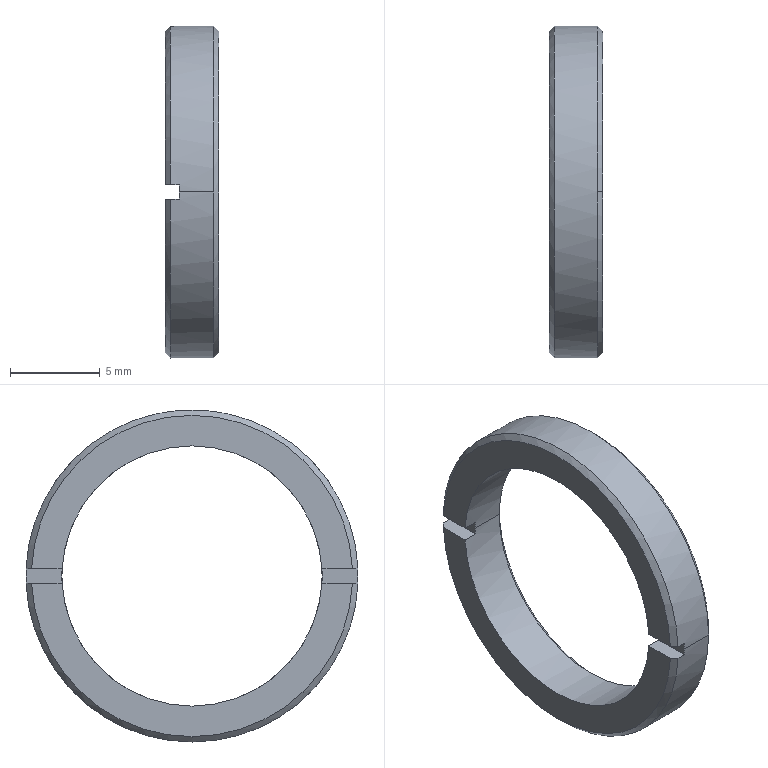Part | STEP file | pressure ring 3.stp.STEP-214.STEP | 1 solid | 20 faces | box 3 x 18.5 x 18.5 mm | volume 301.276 mm3 | plane 9 | cone 7 | cylinder 4 | commonest cylinder face diameters 14.5 x2 18.5 x2
STEP:
#1=CARTESIAN_POINT('',(427.54,0.,7.25));
#2=VERTEX_POINT('',#1);
#3=CARTESIAN_POINT('',(427.54,-7.25,0.));
#4=VERTEX_POINT('',#3);
#5=CARTESIAN_POINT('',(427.54,0.,0.));
#6=DIRECTION('',(1.,0.,0.));
#7=DIRECTION('',(0.,0.,1.));
#8=AXIS2_PLACEMENT_3D('',#5,#6,#7);
#9=CIRCLE('',#8,7.25);
#10=EDGE_CURVE('',#2,#4,#9,.T.);
#11=ORIENTED_EDGE('',*,*,#10,.T.);
#12=CARTESIAN_POINT('',(425.64,-7.25,0.));
#13=VERTEX_POINT('',#12);
#14=CARTESIAN_POINT('',(0.,-7.25,0.));
#15=DIRECTION('',(-1.,0.,0.));
#16=VECTOR('',#15,1000.);
#17=LINE('',#14,#16);
#18=EDGE_CURVE('',#4,#13,#17,.T.);
#19=ORIENTED_EDGE('',*,*,#18,.T.);
#20=CARTESIAN_POINT('',(425.64,-7.239,0.4));
#21=VERTEX_POINT('',#20);
#22=CARTESIAN_POINT('',(425.64,0.,0.));
#23=DIRECTION('',(-1.,0.,0.));
#24=DIRECTION('',(0.,0.,-1.));
#25=AXIS2_PLACEMENT_3D('',#22,#23,#24);
#26=CIRCLE('',#25,7.25);
#27=EDGE_CURVE('',#13,#21,#26,.T.);
#28=ORIENTED_EDGE('',*,*,#27,.T.);
#29=CARTESIAN_POINT('',(424.84,-7.239,0.4));
#30=VERTEX_POINT('',#29);
#31=CARTESIAN_POINT('',(0.,-7.239,0.4));
#32=DIRECTION('',(1.,0.,0.));
#33=VECTOR('',#32,1000.);
#34=LINE('',#31,#33);
#35=EDGE_CURVE('',#30,#21,#34,.T.);
#36=ORIENTED_EDGE('',*,*,#35,.F.);
#37=CARTESIAN_POINT('',(424.84,7.239,0.4));
#38=VERTEX_POINT('',#37);
#39=CARTESIAN_POINT('',(424.84,0.,0.));
#40=DIRECTION('',(-1.,0.,0.));
#41=DIRECTION('',(0.,1.,0.));
#42=AXIS2_PLACEMENT_3D('',#39,#40,#41);
#43=CIRCLE('',#42,7.25);
#44=EDGE_CURVE('',#30,#38,#43,.T.);
#45=ORIENTED_EDGE('',*,*,#44,.T.);
#46=CARTESIAN_POINT('',(425.64,7.239,0.4));
#47=VERTEX_POINT('',#46);
#48=CARTESIAN_POINT('',(0.,7.239,0.4));
#49=DIRECTION('',(-1.,0.,0.));
#50=VECTOR('',#49,1000.);
#51=LINE('',#48,#50);
#52=EDGE_CURVE('',#47,#38,#51,.T.);
#53=ORIENTED_EDGE('',*,*,#52,.F.);
#54=CARTESIAN_POINT('',(425.64,7.25,0.));
#55=VERTEX_POINT('',#54);
#56=CARTESIAN_POINT('',(425.64,0.,0.));
#57=DIRECTION('',(-1.,0.,0.));
#58=DIRECTION('',(0.,0.,-1.));
#59=AXIS2_PLACEMENT_3D('',#56,#57,#58);
#60=CIRCLE('',#59,7.25);
#61=EDGE_CURVE('',#47,#55,#60,.T.);
#62=ORIENTED_EDGE('',*,*,#61,.T.);
#63=CARTESIAN_POINT('',(427.54,7.25,0.));
#64=VERTEX_POINT('',#63);
#65=CARTESIAN_POINT('',(0.,7.25,0.));
#66=DIRECTION('',(-1.,0.,0.));
#67=VECTOR('',#66,1000.);
#68=LINE('',#65,#67);
#69=EDGE_CURVE('',#64,#55,#68,.T.);
#70=ORIENTED_EDGE('',*,*,#69,.F.);
#71=CARTESIAN_POINT('',(427.54,0.,0.));
#72=DIRECTION('',(1.,0.,0.));
#73=DIRECTION('',(0.,0.,1.));
#74=AXIS2_PLACEMENT_3D('',#71,#72,#73);
#75=CIRCLE('',#74,7.25);
#76=EDGE_CURVE('',#64,#2,#75,.T.);
#77=ORIENTED_EDGE('',*,*,#76,.T.);
#78=EDGE_LOOP('',(#11,#19,#28,#36,#45,#53,#62,#70,#77));
#79=FACE_OUTER_BOUND('',#78,.T.);
#80=CARTESIAN_POINT('',(0.,0.,0.));
#81=DIRECTION('',(-1.,0.,0.));
#82=DIRECTION('',(0.,1.,0.));
#83=AXIS2_PLACEMENT_3D('',#80,#81,#82);
#84=CYLINDRICAL_SURFACE('',#83,7.25);
#85=ADVANCED_FACE('',(#79),#84,.F.);
#86=CARTESIAN_POINT('',(427.54,0.,-9.25));
#87=VERTEX_POINT('',#86);
#88=CARTESIAN_POINT('',(427.54,-9.25,0.));
#89=VERTEX_POINT('',#88);
#90=CARTESIAN_POINT('',(427.54,0.,0.));
#91=DIRECTION('',(-1.,0.,0.));
#92=DIRECTION('',(0.,0.,1.));
#93=AXIS2_PLACEMENT_3D('',#90,#91,#92);
#94=CIRCLE('',#93,9.25);
#95=EDGE_CURVE('',#87,#89,#94,.T.);
#96=ORIENTED_EDGE('',*,*,#95,.T.);
#97=CARTESIAN_POINT('',(425.64,-9.25,0.));
#98=VERTEX_POINT('',#97);
#99=CARTESIAN_POINT('',(0.,-9.25,0.));
#100=DIRECTION('',(-1.,0.,0.));
#101=VECTOR('',#100,1000.);
#102=LINE('',#99,#101);
#103=EDGE_CURVE('',#89,#98,#102,.T.);
#104=ORIENTED_EDGE('',*,*,#103,.T.);
#105=CARTESIAN_POINT('',(425.64,-9.241,-0.4));
#106=VERTEX_POINT('',#105);
#107=CARTESIAN_POINT('',(425.64,0.,0.));
#108=DIRECTION('',(1.,0.,0.));
#109=DIRECTION('',(0.,0.,-1.));
#110=AXIS2_PLACEMENT_3D('',#107,#108,#109);
#111=CIRCLE('',#110,9.25);
#112=EDGE_CURVE('',#98,#106,#111,.T.);
#113=ORIENTED_EDGE('',*,*,#112,.T.);
#114=CARTESIAN_POINT('',(425.14,-9.241,-0.4));
#115=VERTEX_POINT('',#114);
#116=CARTESIAN_POINT('',(0.,-9.241,-0.4));
#117=DIRECTION('',(1.,0.,0.));
#118=VECTOR('',#117,1000.);
#119=LINE('',#116,#118);
#120=EDGE_CURVE('',#115,#106,#119,.T.);
#121=ORIENTED_EDGE('',*,*,#120,.F.);
#122=CARTESIAN_POINT('',(425.14,0.,-9.25));
#123=VERTEX_POINT('',#122);
#124=CARTESIAN_POINT('',(425.14,0.,0.));
#125=DIRECTION('',(1.,0.,0.));
#126=DIRECTION('',(0.,0.,-1.));
#127=AXIS2_PLACEMENT_3D('',#124,#125,#126);
#128=CIRCLE('',#127,9.25);
#129=EDGE_CURVE('',#115,#123,#128,.T.);
#130=ORIENTED_EDGE('',*,*,#129,.T.);
#131=CARTESIAN_POINT('',(425.14,9.241,-0.4));
#132=VERTEX_POINT('',#131);
#133=CARTESIAN_POINT('',(425.14,0.,0.));
#134=DIRECTION('',(1.,0.,0.));
#135=DIRECTION('',(0.,0.,-1.));
#136=AXIS2_PLACEMENT_3D('',#133,#134,#135);
#137=CIRCLE('',#136,9.25);
#138=EDGE_CURVE('',#123,#132,#137,.T.);
#139=ORIENTED_EDGE('',*,*,#138,.T.);
#140=CARTESIAN_POINT('',(425.64,9.241,-0.4));
#141=VERTEX_POINT('',#140);
#142=CARTESIAN_POINT('',(0.,9.241,-0.4));
#143=DIRECTION('',(-1.,0.,0.));
#144=VECTOR('',#143,1000.);
#145=LINE('',#142,#144);
#146=EDGE_CURVE('',#141,#132,#145,.T.);
#147=ORIENTED_EDGE('',*,*,#146,.F.);
#148=CARTESIAN_POINT('',(425.64,9.25,0.));
#149=VERTEX_POINT('',#148);
#150=CARTESIAN_POINT('',(425.64,0.,0.));
#151=DIRECTION('',(1.,0.,0.));
#152=DIRECTION('',(0.,0.,-1.));
#153=AXIS2_PLACEMENT_3D('',#150,#151,#152);
#154=CIRCLE('',#153,9.25);
#155=EDGE_CURVE('',#141,#149,#154,.T.);
#156=ORIENTED_EDGE('',*,*,#155,.T.);
#157=CARTESIAN_POINT('',(427.54,9.25,0.));
#158=VERTEX_POINT('',#157);
#159=CARTESIAN_POINT('',(0.,9.25,0.));
#160=DIRECTION('',(-1.,0.,0.));
#161=VECTOR('',#160,1000.);
#162=LINE('',#159,#161);
#163=EDGE_CURVE('',#158,#149,#162,.T.);
#164=ORIENTED_EDGE('',*,*,#163,.F.);
#165=CARTESIAN_POINT('',(427.54,0.,0.));
#166=DIRECTION('',(-1.,0.,0.));
#167=DIRECTION('',(0.,0.,1.));
#168=AXIS2_PLACEMENT_3D('',#165,#166,#167);
#169=CIRCLE('',#168,9.25);
#170=EDGE_CURVE('',#158,#87,#169,.T.);
#171=ORIENTED_EDGE('',*,*,#170,.T.);
#172=EDGE_LOOP('',(#96,#104,#113,#121,#130,#139,#147,#156,#164,#171));
#173=FACE_OUTER_BOUND('',#172,.T.);
#174=CARTESIAN_POINT('',(0.,0.,0.));
#175=DIRECTION('',(-1.,0.,0.));
#176=DIRECTION('',(0.,1.,0.));
#177=AXIS2_PLACEMENT_3D('',#174,#175,#176);
#178=CYLINDRICAL_SURFACE('',#177,9.25);
#179=ADVANCED_FACE('',(#173),#178,.T.);
#180=ORIENTED_EDGE('',*,*,#10,.F.);
#181=CARTESIAN_POINT('',(427.84,0.,7.55));
#182=VERTEX_POINT('',#181);
#183=CARTESIAN_POINT('',(427.84,0.,7.55));
#184=DIRECTION('',(0.7071,0.,0.7071));
#185=VECTOR('',#184,1000.);
#186=LINE('',#183,#185);
#187=EDGE_CURVE('',#2,#182,#186,.T.);
#188=ORIENTED_EDGE('',*,*,#187,.T.);
#189=CARTESIAN_POINT('',(427.84,0.,-7.55));
#190=VERTEX_POINT('',#189);
#191=CARTESIAN_POINT('',(427.84,0.,0.));
#192=DIRECTION('',(-1.,0.,0.));
#193=DIRECTION('',(0.,0.,1.));
#194=AXIS2_PLACEMENT_3D('',#191,#192,#193);
#195=CIRCLE('',#194,7.55);
#196=EDGE_CURVE('',#190,#182,#195,.T.);
#197=ORIENTED_EDGE('',*,*,#196,.F.);
#198=CARTESIAN_POINT('',(427.54,0.,-7.25));
#199=VERTEX_POINT('',#198);
#200=CARTESIAN_POINT('',(427.84,0.,-7.55));
#201=DIRECTION('',(0.7071,0.,-0.7071));
#202=VECTOR('',#201,1000.);
#203=LINE('',#200,#202);
#204=EDGE_CURVE('',#199,#190,#203,.T.);
#205=ORIENTED_EDGE('',*,*,#204,.F.);
#206=CARTESIAN_POINT('',(427.54,0.,0.));
#207=DIRECTION('',(1.,0.,0.));
#208=DIRECTION('',(0.,0.,1.));
#209=AXIS2_PLACEMENT_3D('',#206,#207,#208);
#210=CIRCLE('',#209,7.25);
#211=EDGE_CURVE('',#4,#199,#210,.T.);
#212=ORIENTED_EDGE('',*,*,#211,.F.);
#213=EDGE_LOOP('',(#180,#188,#197,#205,#212));
#214=FACE_OUTER_BOUND('',#213,.T.);
#215=CARTESIAN_POINT('',(427.84,0.,0.));
#216=DIRECTION('',(1.,0.,0.));
#217=DIRECTION('',(0.,0.,-1.));
#218=AXIS2_PLACEMENT_3D('',#215,#216,#217);
#219=CONICAL_SURFACE('',#218,7.55,0.7854);
#220=ADVANCED_FACE('',(#214),#219,.F.);
#221=CARTESIAN_POINT('',(424.84,0.,-8.95));
#222=VERTEX_POINT('',#221);
#223=CARTESIAN_POINT('',(424.84,-8.941,-0.4));
#224=VERTEX_POINT('',#223);
#225=CARTESIAN_POINT('',(424.84,0.,0.));
#226=DIRECTION('',(-1.,0.,0.));
#227=DIRECTION('',(0.,0.,-1.));
#228=AXIS2_PLACEMENT_3D('',#225,#226,#227);
#229=CIRCLE('',#228,8.95);
#230=EDGE_CURVE('',#222,#224,#229,.T.);
#231=ORIENTED_EDGE('',*,*,#230,.F.);
#232=CARTESIAN_POINT('',(424.84,0.,-8.95));
#233=DIRECTION('',(0.7071,0.,-0.7071));
#234=VECTOR('',#233,1000.);
#235=LINE('',#232,#234);
#236=EDGE_CURVE('',#222,#123,#235,.T.);
#237=ORIENTED_EDGE('',*,*,#236,.T.);
#238=ORIENTED_EDGE('',*,*,#129,.F.);
#239=CARTESIAN_POINT('',(424.84,-8.941,-0.4));
#240=CARTESIAN_POINT('',(424.94,-9.041,-0.4));
#241=CARTESIAN_POINT('',(425.04,-9.141,-0.4));
#242=CARTESIAN_POINT('',(425.14,-9.241,-0.4));
#243=B_SPLINE_CURVE_WITH_KNOTS('',3,(#239,#240,#241,#242),.UNSPECIFIED.,.F.,.F.,(4,4),(0.,0.0004245),.UNSPECIFIED.);
#244=EDGE_CURVE('',#224,#115,#243,.T.);
#245=ORIENTED_EDGE('',*,*,#244,.F.);
#246=EDGE_LOOP('',(#231,#237,#238,#245));
#247=FACE_OUTER_BOUND('',#246,.T.);
#248=CARTESIAN_POINT('',(424.84,0.,0.));
#249=DIRECTION('',(1.,0.,0.));
#250=DIRECTION('',(0.,0.,-1.));
#251=AXIS2_PLACEMENT_3D('',#248,#249,#250);
#252=CONICAL_SURFACE('',#251,8.95,0.7854);
#253=ADVANCED_FACE('',(#247),#252,.T.);
#254=CARTESIAN_POINT('',(427.84,0.,-8.95));
#255=VERTEX_POINT('',#254);
#256=CARTESIAN_POINT('',(427.84,0.,8.95));
#257=VERTEX_POINT('',#256);
#258=CARTESIAN_POINT('',(427.84,0.,0.));
#259=DIRECTION('',(1.,0.,0.));
#260=DIRECTION('',(0.,0.,1.));
#261=AXIS2_PLACEMENT_3D('',#258,#259,#260);
#262=CIRCLE('',#261,8.95);
#263=EDGE_CURVE('',#255,#257,#262,.T.);
#264=ORIENTED_EDGE('',*,*,#263,.F.);
#265=CARTESIAN_POINT('',(427.54,0.,-9.25));
#266=DIRECTION('',(-0.7071,0.,-0.7071));
#267=VECTOR('',#266,1000.);
#268=LINE('',#265,#267);
#269=EDGE_CURVE('',#255,#87,#268,.T.);
#270=ORIENTED_EDGE('',*,*,#269,.T.);
#271=ORIENTED_EDGE('',*,*,#170,.F.);
#272=CARTESIAN_POINT('',(427.54,0.,9.25));
#273=VERTEX_POINT('',#272);
#274=CARTESIAN_POINT('',(427.54,0.,0.));
#275=DIRECTION('',(-1.,0.,0.));
#276=DIRECTION('',(0.,0.,1.));
#277=AXIS2_PLACEMENT_3D('',#274,#275,#276);
#278=CIRCLE('',#277,9.25);
#279=EDGE_CURVE('',#273,#158,#278,.T.);
#280=ORIENTED_EDGE('',*,*,#279,.F.);
#281=CARTESIAN_POINT('',(427.54,0.,9.25));
#282=DIRECTION('',(-0.7071,0.,0.7071));
#283=VECTOR('',#282,1000.);
#284=LINE('',#281,#283);
#285=EDGE_CURVE('',#257,#273,#284,.T.);
#286=ORIENTED_EDGE('',*,*,#285,.F.);
#287=EDGE_LOOP('',(#264,#270,#271,#280,#286));
#288=FACE_OUTER_BOUND('',#287,.T.);
#289=CARTESIAN_POINT('',(427.54,0.,0.));
#290=DIRECTION('',(-1.,0.,0.));
#291=DIRECTION('',(0.,0.,1.));
#292=AXIS2_PLACEMENT_3D('',#289,#290,#291);
#293=CONICAL_SURFACE('',#292,9.25,0.7854);
#294=ADVANCED_FACE('',(#288),#293,.T.);
#295=ORIENTED_EDGE('',*,*,#269,.F.);
#296=CARTESIAN_POINT('',(427.84,0.,0.));
#297=DIRECTION('',(1.,0.,0.));
#298=DIRECTION('',(0.,0.,1.));
#299=AXIS2_PLACEMENT_3D('',#296,#297,#298);
#300=CIRCLE('',#299,8.95);
#301=EDGE_CURVE('',#257,#255,#300,.T.);
#302=ORIENTED_EDGE('',*,*,#301,.F.);
#303=ORIENTED_EDGE('',*,*,#285,.T.);
#304=CARTESIAN_POINT('',(427.54,0.,0.));
#305=DIRECTION('',(-1.,0.,0.));
#306=DIRECTION('',(0.,0.,1.));
#307=AXIS2_PLACEMENT_3D('',#304,#305,#306);
#308=CIRCLE('',#307,9.25);
#309=EDGE_CURVE('',#89,#273,#308,.T.);
#310=ORIENTED_EDGE('',*,*,#309,.F.);
#311=ORIENTED_EDGE('',*,*,#95,.F.);
#312=EDGE_LOOP('',(#295,#302,#303,#310,#311));
#313=FACE_OUTER_BOUND('',#312,.T.);
#314=CARTESIAN_POINT('',(427.54,0.,0.));
#315=DIRECTION('',(-1.,0.,0.));
#316=DIRECTION('',(0.,0.,1.));
#317=AXIS2_PLACEMENT_3D('',#314,#315,#316);
#318=CONICAL_SURFACE('',#317,9.25,0.7854);
#319=ADVANCED_FACE('',(#313),#318,.T.);
#320=ORIENTED_EDGE('',*,*,#236,.F.);
#321=CARTESIAN_POINT('',(424.84,8.941,-0.4));
#322=VERTEX_POINT('',#321);
#323=CARTESIAN_POINT('',(424.84,0.,0.));
#324=DIRECTION('',(-1.,0.,0.));
#325=DIRECTION('',(0.,0.,-1.));
#326=AXIS2_PLACEMENT_3D('',#323,#324,#325);
#327=CIRCLE('',#326,8.95);
#328=EDGE_CURVE('',#322,#222,#327,.T.);
#329=ORIENTED_EDGE('',*,*,#328,.F.);
#330=CARTESIAN_POINT('',(425.14,9.241,-0.4));
#331=CARTESIAN_POINT('',(425.04,9.141,-0.4));
#332=CARTESIAN_POINT('',(424.94,9.041,-0.4));
#333=CARTESIAN_POINT('',(424.84,8.941,-0.4));
#334=B_SPLINE_CURVE_WITH_KNOTS('',3,(#330,#331,#332,#333),.UNSPECIFIED.,.F.,.F.,(4,4),(0.,0.0004245),.UNSPECIFIED.);
#335=EDGE_CURVE('',#132,#322,#334,.T.);
#336=ORIENTED_EDGE('',*,*,#335,.F.);
#337=ORIENTED_EDGE('',*,*,#138,.F.);
#338=EDGE_LOOP('',(#320,#329,#336,#337));
#339=FACE_OUTER_BOUND('',#338,.T.);
#340=CARTESIAN_POINT('',(424.84,0.,0.));
#341=DIRECTION('',(1.,0.,0.));
#342=DIRECTION('',(0.,0.,-1.));
#343=AXIS2_PLACEMENT_3D('',#340,#341,#342);
#344=CONICAL_SURFACE('',#343,8.95,0.7854);
#345=ADVANCED_FACE('',(#339),#344,.T.);
#346=CARTESIAN_POINT('',(424.84,-8.941,0.4));
#347=VERTEX_POINT('',#346);
#348=CARTESIAN_POINT('',(424.84,-10.,0.4));
#349=DIRECTION('',(0.,1.,0.));
#350=VECTOR('',#349,1000.);
#351=LINE('',#348,#350);
#352=EDGE_CURVE('',#347,#30,#351,.T.);
#353=ORIENTED_EDGE('',*,*,#352,.F.);
#354=CARTESIAN_POINT('',(424.84,8.941,0.4));
#355=VERTEX_POINT('',#354);
#356=CARTESIAN_POINT('',(424.84,0.,0.));
#357=DIRECTION('',(-1.,0.,0.));
#358=DIRECTION('',(0.,0.,-1.));
#359=AXIS2_PLACEMENT_3D('',#356,#357,#358);
#360=CIRCLE('',#359,8.95);
#361=EDGE_CURVE('',#347,#355,#360,.T.);
#362=ORIENTED_EDGE('',*,*,#361,.T.);
#363=CARTESIAN_POINT('',(424.84,-10.,0.4));
#364=DIRECTION('',(0.,1.,0.));
#365=VECTOR('',#364,1000.);
#366=LINE('',#363,#365);
#367=EDGE_CURVE('',#38,#355,#366,.T.);
#368=ORIENTED_EDGE('',*,*,#367,.F.);
#369=ORIENTED_EDGE('',*,*,#44,.F.);
#370=EDGE_LOOP('',(#353,#362,#368,#369));
#371=FACE_OUTER_BOUND('',#370,.T.);
#372=CARTESIAN_POINT('',(424.84,9.25,0.));
#373=DIRECTION('',(1.,0.,0.));
#374=DIRECTION('',(0.,1.,0.));
#375=AXIS2_PLACEMENT_3D('',#372,#373,#374);
#376=PLANE('',#375);
#377=ADVANCED_FACE('',(#371),#376,.F.);
#378=CARTESIAN_POINT('',(424.84,-7.239,-0.4));
#379=VERTEX_POINT('',#378);
#380=CARTESIAN_POINT('',(424.84,10.,-0.4));
#381=DIRECTION('',(0.,-1.,0.));
#382=VECTOR('',#381,1000.);
#383=LINE('',#380,#382);
#384=EDGE_CURVE('',#379,#224,#383,.T.);
#385=ORIENTED_EDGE('',*,*,#384,.T.);
#386=ORIENTED_EDGE('',*,*,#244,.T.);
#387=ORIENTED_EDGE('',*,*,#120,.T.);
#388=CARTESIAN_POINT('',(425.64,-7.239,-0.4));
#389=VERTEX_POINT('',#388);
#390=CARTESIAN_POINT('',(425.64,10.,-0.4));
#391=DIRECTION('',(0.,-1.,0.));
#392=VECTOR('',#391,1000.);
#393=LINE('',#390,#392);
#394=EDGE_CURVE('',#389,#106,#393,.T.);
#395=ORIENTED_EDGE('',*,*,#394,.F.);
#396=CARTESIAN_POINT('',(0.,-7.239,-0.4));
#397=DIRECTION('',(-1.,0.,0.));
#398=VECTOR('',#397,1000.);
#399=LINE('',#396,#398);
#400=EDGE_CURVE('',#389,#379,#399,.T.);
#401=ORIENTED_EDGE('',*,*,#400,.T.);
#402=EDGE_LOOP('',(#385,#386,#387,#395,#401));
#403=FACE_OUTER_BOUND('',#402,.T.);
#404=CARTESIAN_POINT('',(425.64,10.,-0.4));
#405=DIRECTION('',(0.,0.,1.));
#406=DIRECTION('',(0.,-1.,0.));
#407=AXIS2_PLACEMENT_3D('',#404,#405,#406);
#408=PLANE('',#407);
#409=ADVANCED_FACE('',(#403),#408,.T.);
#410=CARTESIAN_POINT('',(425.64,-9.241,0.4));
#411=VERTEX_POINT('',#410);
#412=CARTESIAN_POINT('',(425.14,-9.241,0.4));
#413=VERTEX_POINT('',#412);
#414=CARTESIAN_POINT('',(0.,-9.241,0.4));
#415=DIRECTION('',(-1.,0.,0.));
#416=VECTOR('',#415,1000.);
#417=LINE('',#414,#416);
#418=EDGE_CURVE('',#411,#413,#417,.T.);
#419=ORIENTED_EDGE('',*,*,#418,.T.);
#420=CARTESIAN_POINT('',(425.14,-9.241,0.4));
#421=CARTESIAN_POINT('',(425.04,-9.141,0.4));
#422=CARTESIAN_POINT('',(424.94,-9.041,0.4));
#423=CARTESIAN_POINT('',(424.84,-8.941,0.4));
#424=B_SPLINE_CURVE_WITH_KNOTS('',3,(#420,#421,#422,#423),.UNSPECIFIED.,.F.,.F.,(4,4),(0.,0.0004245),.UNSPECIFIED.);
#425=EDGE_CURVE('',#413,#347,#424,.T.);
#426=ORIENTED_EDGE('',*,*,#425,.T.);
#427=ORIENTED_EDGE('',*,*,#352,.T.);
#428=ORIENTED_EDGE('',*,*,#35,.T.);
#429=CARTESIAN_POINT('',(425.64,-10.,0.4));
#430=DIRECTION('',(0.,1.,0.));
#431=VECTOR('',#430,1000.);
#432=LINE('',#429,#431);
#433=EDGE_CURVE('',#411,#21,#432,.T.);
#434=ORIENTED_EDGE('',*,*,#433,.F.);
#435=EDGE_LOOP('',(#419,#426,#427,#428,#434));
#436=FACE_OUTER_BOUND('',#435,.T.);
#437=CARTESIAN_POINT('',(425.64,-10.,0.4));
#438=DIRECTION('',(0.,0.,-1.));
#439=DIRECTION('',(0.,-1.,0.));
#440=AXIS2_PLACEMENT_3D('',#437,#438,#439);
#441=PLANE('',#440);
#442=ADVANCED_FACE('',(#436),#441,.T.);
#443=ORIENTED_EDGE('',*,*,#367,.T.);
#444=CARTESIAN_POINT('',(425.14,9.241,0.4));
#445=VERTEX_POINT('',#444);
#446=CARTESIAN_POINT('',(424.84,8.941,0.4));
#447=CARTESIAN_POINT('',(424.94,9.041,0.4));
#448=CARTESIAN_POINT('',(425.04,9.141,0.4));
#449=CARTESIAN_POINT('',(425.14,9.241,0.4));
#450=B_SPLINE_CURVE_WITH_KNOTS('',3,(#446,#447,#448,#449),.UNSPECIFIED.,.F.,.F.,(4,4),(0.,0.0004245),.UNSPECIFIED.);
#451=EDGE_CURVE('',#355,#445,#450,.T.);
#452=ORIENTED_EDGE('',*,*,#451,.T.);
#453=CARTESIAN_POINT('',(425.64,9.241,0.4));
#454=VERTEX_POINT('',#453);
#455=CARTESIAN_POINT('',(0.,9.241,0.4));
#456=DIRECTION('',(1.,0.,0.));
#457=VECTOR('',#456,1000.);
#458=LINE('',#455,#457);
#459=EDGE_CURVE('',#445,#454,#458,.T.);
#460=ORIENTED_EDGE('',*,*,#459,.T.);
#461=CARTESIAN_POINT('',(425.64,-10.,0.4));
#462=DIRECTION('',(0.,1.,0.));
#463=VECTOR('',#462,1000.);
#464=LINE('',#461,#463);
#465=EDGE_CURVE('',#47,#454,#464,.T.);
#466=ORIENTED_EDGE('',*,*,#465,.F.);
#467=ORIENTED_EDGE('',*,*,#52,.T.);
#468=EDGE_LOOP('',(#443,#452,#460,#466,#467));
#469=FACE_OUTER_BOUND('',#468,.T.);
#470=CARTESIAN_POINT('',(425.64,-10.,0.4));
#471=DIRECTION('',(0.,0.,-1.));
#472=DIRECTION('',(0.,-1.,0.));
#473=AXIS2_PLACEMENT_3D('',#470,#471,#472);
#474=PLANE('',#473);
#475=ADVANCED_FACE('',(#469),#474,.T.);
#476=ORIENTED_EDGE('',*,*,#433,.T.);
#477=ORIENTED_EDGE('',*,*,#27,.F.);
#478=CARTESIAN_POINT('',(425.64,0.,0.));
#479=DIRECTION('',(-1.,0.,0.));
#480=DIRECTION('',(0.,0.,-1.));
#481=AXIS2_PLACEMENT_3D('',#478,#479,#480);
#482=CIRCLE('',#481,7.25);
#483=EDGE_CURVE('',#389,#13,#482,.T.);
#484=ORIENTED_EDGE('',*,*,#483,.F.);
#485=ORIENTED_EDGE('',*,*,#394,.T.);
#486=ORIENTED_EDGE('',*,*,#112,.F.);
#487=CARTESIAN_POINT('',(425.64,0.,0.));
#488=DIRECTION('',(1.,0.,0.));
#489=DIRECTION('',(0.,0.,-1.));
#490=AXIS2_PLACEMENT_3D('',#487,#488,#489);
#491=CIRCLE('',#490,9.25);
#492=EDGE_CURVE('',#411,#98,#491,.T.);
#493=ORIENTED_EDGE('',*,*,#492,.F.);
#494=EDGE_LOOP('',(#476,#477,#484,#485,#486,#493));
#495=FACE_OUTER_BOUND('',#494,.T.);
#496=CARTESIAN_POINT('',(425.64,-25.,-25.));
#497=DIRECTION('',(1.,0.,0.));
#498=DIRECTION('',(0.,1.,0.));
#499=AXIS2_PLACEMENT_3D('',#496,#497,#498);
#500=PLANE('',#499);
#501=ADVANCED_FACE('',(#495),#500,.F.);
#502=ORIENTED_EDGE('',*,*,#187,.F.);
#503=ORIENTED_EDGE('',*,*,#76,.F.);
#504=CARTESIAN_POINT('',(427.54,0.,0.));
#505=DIRECTION('',(1.,0.,0.));
#506=DIRECTION('',(0.,0.,1.));
#507=AXIS2_PLACEMENT_3D('',#504,#505,#506);
#508=CIRCLE('',#507,7.25);
#509=EDGE_CURVE('',#199,#64,#508,.T.);
#510=ORIENTED_EDGE('',*,*,#509,.F.);
#511=ORIENTED_EDGE('',*,*,#204,.T.);
#512=CARTESIAN_POINT('',(427.84,0.,0.));
#513=DIRECTION('',(-1.,0.,0.));
#514=DIRECTION('',(0.,0.,1.));
#515=AXIS2_PLACEMENT_3D('',#512,#513,#514);
#516=CIRCLE('',#515,7.55);
#517=EDGE_CURVE('',#182,#190,#516,.T.);
#518=ORIENTED_EDGE('',*,*,#517,.F.);
#519=EDGE_LOOP('',(#502,#503,#510,#511,#518));
#520=FACE_OUTER_BOUND('',#519,.T.);
#521=CARTESIAN_POINT('',(427.84,0.,0.));
#522=DIRECTION('',(1.,0.,0.));
#523=DIRECTION('',(0.,0.,-1.));
#524=AXIS2_PLACEMENT_3D('',#521,#522,#523);
#525=CONICAL_SURFACE('',#524,7.55,0.7854);
#526=ADVANCED_FACE('',(#520),#525,.F.);
#527=CARTESIAN_POINT('',(425.64,7.239,-0.4));
#528=VERTEX_POINT('',#527);
#529=CARTESIAN_POINT('',(425.64,10.,-0.4));
#530=DIRECTION('',(0.,-1.,0.));
#531=VECTOR('',#530,1000.);
#532=LINE('',#529,#531);
#533=EDGE_CURVE('',#141,#528,#532,.T.);
#534=ORIENTED_EDGE('',*,*,#533,.T.);
#535=CARTESIAN_POINT('',(425.64,0.,0.));
#536=DIRECTION('',(-1.,0.,0.));
#537=DIRECTION('',(0.,0.,-1.));
#538=AXIS2_PLACEMENT_3D('',#535,#536,#537);
#539=CIRCLE('',#538,7.25);
#540=EDGE_CURVE('',#55,#528,#539,.T.);
#541=ORIENTED_EDGE('',*,*,#540,.F.);
#542=ORIENTED_EDGE('',*,*,#61,.F.);
#543=ORIENTED_EDGE('',*,*,#465,.T.);
#544=CARTESIAN_POINT('',(425.64,0.,0.));
#545=DIRECTION('',(1.,0.,0.));
#546=DIRECTION('',(0.,0.,-1.));
#547=AXIS2_PLACEMENT_3D('',#544,#545,#546);
#548=CIRCLE('',#547,9.25);
#549=EDGE_CURVE('',#149,#454,#548,.T.);
#550=ORIENTED_EDGE('',*,*,#549,.F.);
#551=ORIENTED_EDGE('',*,*,#155,.F.);
#552=EDGE_LOOP('',(#534,#541,#542,#543,#550,#551));
#553=FACE_OUTER_BOUND('',#552,.T.);
#554=CARTESIAN_POINT('',(425.64,-25.,-25.));
#555=DIRECTION('',(1.,0.,0.));
#556=DIRECTION('',(0.,1.,0.));
#557=AXIS2_PLACEMENT_3D('',#554,#555,#556);
#558=PLANE('',#557);
#559=ADVANCED_FACE('',(#553),#558,.F.);
#560=ORIENTED_EDGE('',*,*,#196,.T.);
#561=ORIENTED_EDGE('',*,*,#517,.T.);
#562=EDGE_LOOP('',(#560,#561));
#563=FACE_BOUND('',#562,.T.);
#564=ORIENTED_EDGE('',*,*,#301,.T.);
#565=ORIENTED_EDGE('',*,*,#263,.T.);
#566=EDGE_LOOP('',(#564,#565));
#567=FACE_OUTER_BOUND('',#566,.T.);
#568=CARTESIAN_POINT('',(427.84,7.25,0.));
#569=DIRECTION('',(-1.,0.,0.));
#570=DIRECTION('',(0.,0.,1.));
#571=AXIS2_PLACEMENT_3D('',#568,#569,#570);
#572=PLANE('',#571);
#573=ADVANCED_FACE('',(#563,#567),#572,.F.);
#574=ORIENTED_EDGE('',*,*,#103,.F.);
#575=ORIENTED_EDGE('',*,*,#309,.T.);
#576=ORIENTED_EDGE('',*,*,#279,.T.);
#577=ORIENTED_EDGE('',*,*,#163,.T.);
#578=ORIENTED_EDGE('',*,*,#549,.T.);
#579=ORIENTED_EDGE('',*,*,#459,.F.);
#580=CARTESIAN_POINT('',(425.14,0.,0.));
#581=DIRECTION('',(1.,0.,0.));
#582=DIRECTION('',(0.,0.,-1.));
#583=AXIS2_PLACEMENT_3D('',#580,#581,#582);
#584=CIRCLE('',#583,9.25);
#585=EDGE_CURVE('',#445,#413,#584,.T.);
#586=ORIENTED_EDGE('',*,*,#585,.T.);
#587=ORIENTED_EDGE('',*,*,#418,.F.);
#588=ORIENTED_EDGE('',*,*,#492,.T.);
#589=EDGE_LOOP('',(#574,#575,#576,#577,#578,#579,#586,#587,#588));
#590=FACE_OUTER_BOUND('',#589,.T.);
#591=CARTESIAN_POINT('',(0.,0.,0.));
#592=DIRECTION('',(-1.,0.,0.));
#593=DIRECTION('',(0.,1.,0.));
#594=AXIS2_PLACEMENT_3D('',#591,#592,#593);
#595=CYLINDRICAL_SURFACE('',#594,9.25);
#596=ADVANCED_FACE('',(#590),#595,.T.);
#597=CARTESIAN_POINT('',(424.84,7.239,-0.4));
#598=VERTEX_POINT('',#597);
#599=CARTESIAN_POINT('',(424.84,10.,-0.4));
#600=DIRECTION('',(0.,-1.,0.));
#601=VECTOR('',#600,1000.);
#602=LINE('',#599,#601);
#603=EDGE_CURVE('',#322,#598,#602,.T.);
#604=ORIENTED_EDGE('',*,*,#603,.F.);
#605=ORIENTED_EDGE('',*,*,#328,.T.);
#606=ORIENTED_EDGE('',*,*,#230,.T.);
#607=ORIENTED_EDGE('',*,*,#384,.F.);
#608=CARTESIAN_POINT('',(424.84,0.,0.));
#609=DIRECTION('',(-1.,0.,0.));
#610=DIRECTION('',(0.,1.,0.));
#611=AXIS2_PLACEMENT_3D('',#608,#609,#610);
#612=CIRCLE('',#611,7.25);
#613=EDGE_CURVE('',#598,#379,#612,.T.);
#614=ORIENTED_EDGE('',*,*,#613,.F.);
#615=EDGE_LOOP('',(#604,#605,#606,#607,#614));
#616=FACE_OUTER_BOUND('',#615,.T.);
#617=CARTESIAN_POINT('',(424.84,9.25,0.));
#618=DIRECTION('',(1.,0.,0.));
#619=DIRECTION('',(0.,1.,0.));
#620=AXIS2_PLACEMENT_3D('',#617,#618,#619);
#621=PLANE('',#620);
#622=ADVANCED_FACE('',(#616),#621,.F.);
#623=ORIENTED_EDGE('',*,*,#18,.F.);
#624=ORIENTED_EDGE('',*,*,#211,.T.);
#625=ORIENTED_EDGE('',*,*,#509,.T.);
#626=ORIENTED_EDGE('',*,*,#69,.T.);
#627=ORIENTED_EDGE('',*,*,#540,.T.);
#628=CARTESIAN_POINT('',(0.,7.239,-0.4));
#629=DIRECTION('',(1.,0.,0.));
#630=VECTOR('',#629,1000.);
#631=LINE('',#628,#630);
#632=EDGE_CURVE('',#598,#528,#631,.T.);
#633=ORIENTED_EDGE('',*,*,#632,.F.);
#634=ORIENTED_EDGE('',*,*,#613,.T.);
#635=ORIENTED_EDGE('',*,*,#400,.F.);
#636=ORIENTED_EDGE('',*,*,#483,.T.);
#637=EDGE_LOOP('',(#623,#624,#625,#626,#627,#633,#634,#635,#636));
#638=FACE_OUTER_BOUND('',#637,.T.);
#639=CARTESIAN_POINT('',(0.,0.,0.));
#640=DIRECTION('',(-1.,0.,0.));
#641=DIRECTION('',(0.,1.,0.));
#642=AXIS2_PLACEMENT_3D('',#639,#640,#641);
#643=CYLINDRICAL_SURFACE('',#642,7.25);
#644=ADVANCED_FACE('',(#638),#643,.F.);
#645=ORIENTED_EDGE('',*,*,#146,.T.);
#646=ORIENTED_EDGE('',*,*,#335,.T.);
#647=ORIENTED_EDGE('',*,*,#603,.T.);
#648=ORIENTED_EDGE('',*,*,#632,.T.);
#649=ORIENTED_EDGE('',*,*,#533,.F.);
#650=EDGE_LOOP('',(#645,#646,#647,#648,#649));
#651=FACE_OUTER_BOUND('',#650,.T.);
#652=CARTESIAN_POINT('',(425.64,10.,-0.4));
#653=DIRECTION('',(0.,0.,1.));
#654=DIRECTION('',(0.,-1.,0.));
#655=AXIS2_PLACEMENT_3D('',#652,#653,#654);
#656=PLANE('',#655);
#657=ADVANCED_FACE('',(#651),#656,.T.);
#658=ORIENTED_EDGE('',*,*,#425,.F.);
#659=ORIENTED_EDGE('',*,*,#585,.F.);
#660=ORIENTED_EDGE('',*,*,#451,.F.);
#661=ORIENTED_EDGE('',*,*,#361,.F.);
#662=EDGE_LOOP('',(#658,#659,#660,#661));
#663=FACE_OUTER_BOUND('',#662,.T.);
#664=CARTESIAN_POINT('',(424.84,0.,0.));
#665=DIRECTION('',(1.,0.,0.));
#666=DIRECTION('',(0.,0.,-1.));
#667=AXIS2_PLACEMENT_3D('',#664,#665,#666);
#668=CONICAL_SURFACE('',#667,8.95,0.7854);
#669=ADVANCED_FACE('',(#663),#668,.T.);
#670=CLOSED_SHELL('',(#85,#179,#220,#253,#294,#319,#345,#377,#409,#442,#475,#501,#526,#559,#573,#596,#622,#644,#657,#669));
#671=MANIFOLD_SOLID_BREP('',#670);
#672=CARTESIAN_POINT('',(0.,0.,0.));
#673=DIRECTION('',(0.,0.,1.));
#674=DIRECTION('',(1.,0.,0.));
#675=AXIS2_PLACEMENT_3D('',#672,#673,#674);
#676=(LENGTH_UNIT()NAMED_UNIT(*)SI_UNIT(.MILLI.,.METRE.));
#677=UNCERTAINTY_MEASURE_WITH_UNIT(LENGTH_MEASURE(0.00001),#676,'','');
#678=(NAMED_UNIT(*)PLANE_ANGLE_UNIT()SI_UNIT($,.RADIAN.));
#679=(NAMED_UNIT(*)SI_UNIT($,.STERADIAN.)SOLID_ANGLE_UNIT());
#680=(GEOMETRIC_REPRESENTATION_CONTEXT(3)GLOBAL_UNCERTAINTY_ASSIGNED_CONTEXT((#677))GLOBAL_UNIT_ASSIGNED_CONTEXT((#676,#678,#679))REPRESENTATION_CONTEXT('',''));
#681=ADVANCED_BREP_SHAPE_REPRESENTATION('',(#671,#675),#680);